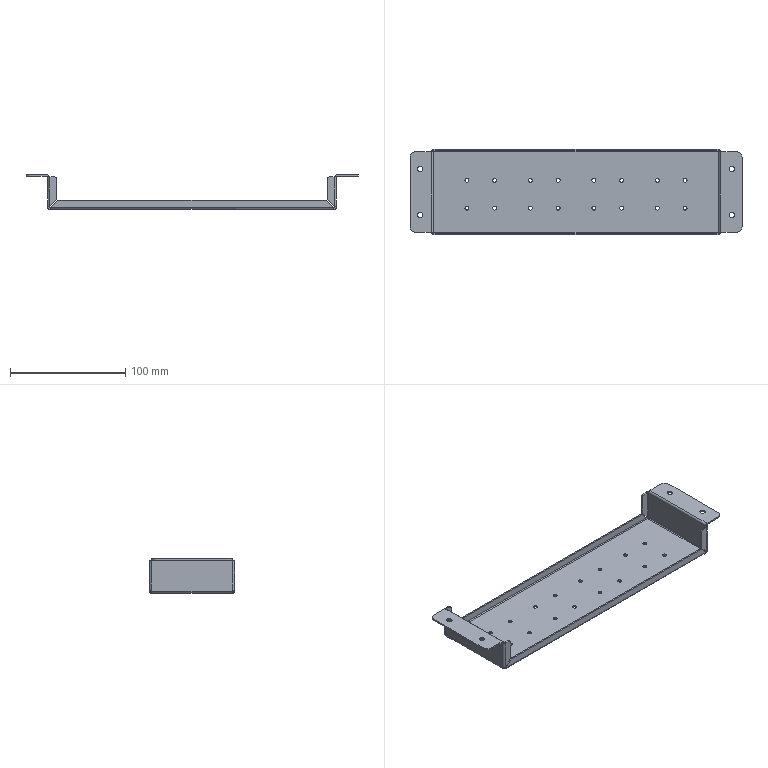Part | SolidWorks | features EdgeFlange 3, Fillet 3, LPattern 2, Cut 1, FlatPattern 1, ICE 1, SMBaseFlange 1, SheetMetal 1 | 1 solid | 134 faces | box 287.6 x 73.8 x 30 mm | volume 34168 mm3 | cylinder 68 | plane 58 | spline 8 | commonest cylinder face diameters 3.4 x34 1.4 x8 3.8 x8 4.5 x8 6 x4 10 x4